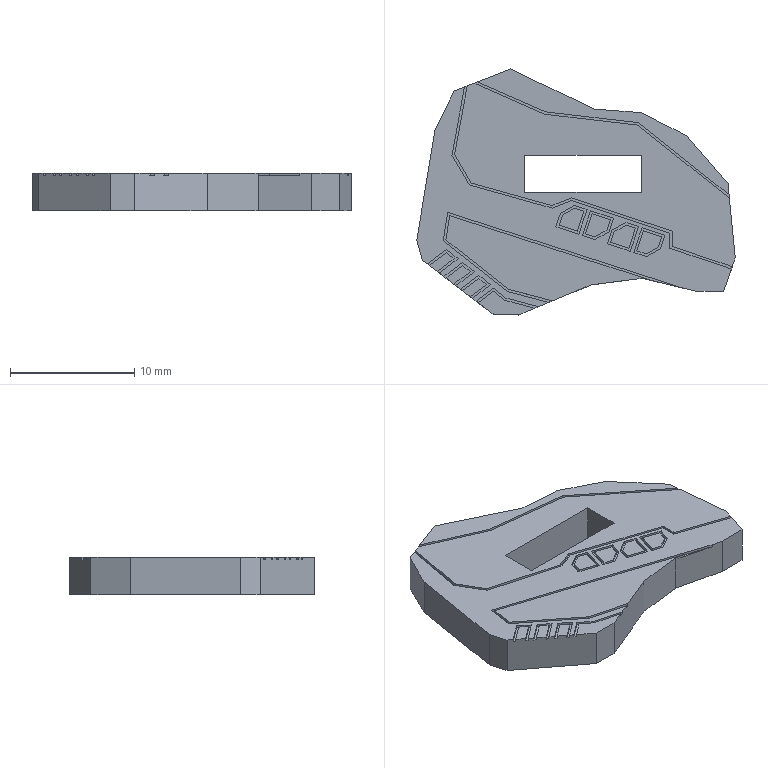Part | SolidWorks | features BaseBody 1 | 1 solid | 136 faces | box 25.647 x 19.802 x 3 mm | volume 997.397 mm3 | plane 120 | spline 16